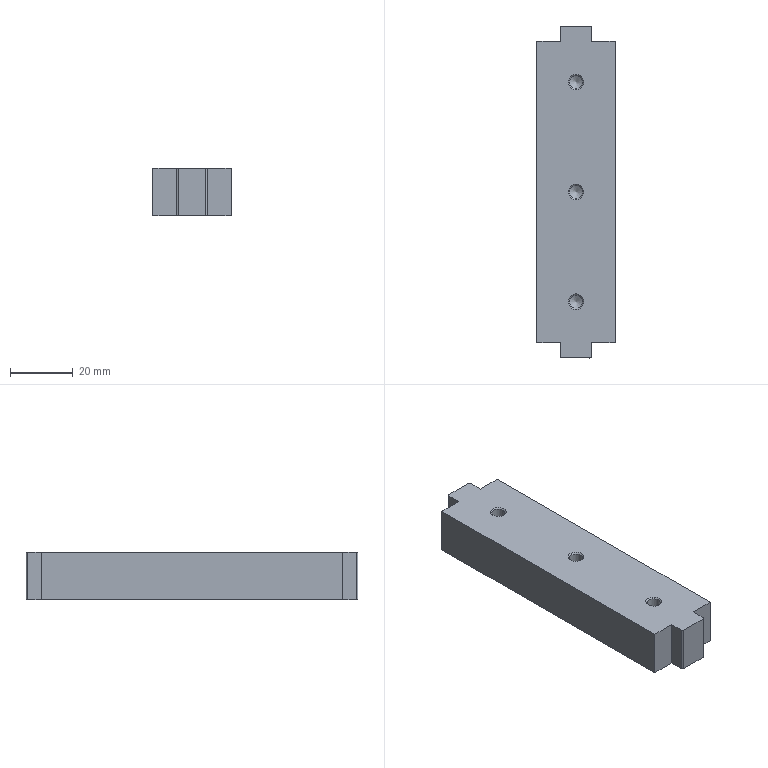Part | STEP file | 200 mesh_id1990 | 1 solid | 27 faces | box 25 x 105.8 x 15 mm | volume 37116 mm3 | plane 14 | cylinder 7 | cone 6 | commonest cylinder face diameters 0.9 x4 4.2 x3
STEP:
#1=CARTESIAN_POINT('',(-17200.384,-3974.819,45.));
#2=VERTEX_POINT('',#1);
#3=CARTESIAN_POINT('',(-17200.384,-4070.819,45.));
#4=VERTEX_POINT('',#3);
#5=CARTESIAN_POINT('',(-17200.384,-4072.469,45.));
#6=DIRECTION('',(0.,-1.,0.));
#7=VECTOR('',#6,1.);
#8=LINE('',#5,#7);
#9=EDGE_CURVE('',#2,#4,#8,.T.);
#10=ORIENTED_EDGE('',*,*,#9,.F.);
#11=CARTESIAN_POINT('',(-17200.384,-3974.819,60.));
#12=VERTEX_POINT('',#11);
#13=CARTESIAN_POINT('',(-17200.384,-3974.819,65.));
#14=DIRECTION('',(0.,0.,-1.));
#15=VECTOR('',#14,1.);
#16=LINE('',#13,#15);
#17=EDGE_CURVE('',#12,#2,#16,.T.);
#18=ORIENTED_EDGE('',*,*,#17,.F.);
#19=CARTESIAN_POINT('',(-17200.384,-4070.819,60.));
#20=VERTEX_POINT('',#19);
#21=CARTESIAN_POINT('',(-17200.384,-3977.669,60.));
#22=DIRECTION('',(0.,-1.,0.));
#23=VECTOR('',#22,1.);
#24=LINE('',#21,#23);
#25=EDGE_CURVE('',#12,#20,#24,.T.);
#26=ORIENTED_EDGE('',*,*,#25,.T.);
#27=CARTESIAN_POINT('',(-17200.384,-4070.819,65.));
#28=DIRECTION('',(0.,0.,-1.));
#29=VECTOR('',#28,1.);
#30=LINE('',#27,#29);
#31=EDGE_CURVE('',#20,#4,#30,.T.);
#32=ORIENTED_EDGE('',*,*,#31,.T.);
#33=EDGE_LOOP('',(#10,#18,#26,#32));
#34=FACE_OUTER_BOUND('',#33,.T.);
#35=CARTESIAN_POINT('',(-17200.384,-3977.669,65.));
#36=DIRECTION('',(1.,0.,0.));
#37=DIRECTION('',(0.,0.,1.));
#38=AXIS2_PLACEMENT_3D('',#35,#36,#37);
#39=PLANE('',#38);
#40=ADVANCED_FACE('',(#34),#39,.T.);
#41=CARTESIAN_POINT('',(-17207.984,-4070.819,45.));
#42=VERTEX_POINT('',#41);
#43=CARTESIAN_POINT('',(-17208.384,-4070.819,45.));
#44=DIRECTION('',(-1.,0.,0.));
#45=VECTOR('',#44,1.);
#46=LINE('',#43,#45);
#47=EDGE_CURVE('',#4,#42,#46,.T.);
#48=ORIENTED_EDGE('',*,*,#47,.F.);
#49=ORIENTED_EDGE('',*,*,#31,.F.);
#50=CARTESIAN_POINT('',(-17207.984,-4070.819,60.));
#51=VERTEX_POINT('',#50);
#52=CARTESIAN_POINT('',(-17208.384,-4070.819,60.));
#53=DIRECTION('',(-1.,0.,0.));
#54=VECTOR('',#53,1.);
#55=LINE('',#52,#54);
#56=EDGE_CURVE('',#20,#51,#55,.T.);
#57=ORIENTED_EDGE('',*,*,#56,.T.);
#58=CARTESIAN_POINT('',(-17207.984,-4070.819,65.));
#59=DIRECTION('',(0.,0.,-1.));
#60=VECTOR('',#59,1.);
#61=LINE('',#58,#60);
#62=EDGE_CURVE('',#51,#42,#61,.T.);
#63=ORIENTED_EDGE('',*,*,#62,.T.);
#64=EDGE_LOOP('',(#48,#49,#57,#63));
#65=FACE_OUTER_BOUND('',#64,.T.);
#66=CARTESIAN_POINT('',(-17200.384,-4070.819,65.));
#67=DIRECTION('',(0.,-1.,0.));
#68=DIRECTION('',(0.,0.,1.));
#69=AXIS2_PLACEMENT_3D('',#66,#67,#68);
#70=PLANE('',#69);
#71=ADVANCED_FACE('',(#65),#70,.T.);
#72=CARTESIAN_POINT('',(-17207.984,-4075.269,45.));
#73=VERTEX_POINT('',#72);
#74=CARTESIAN_POINT('',(-17207.984,-4075.369,45.));
#75=DIRECTION('',(0.,-1.,0.));
#76=VECTOR('',#75,1.);
#77=LINE('',#74,#76);
#78=EDGE_CURVE('',#42,#73,#77,.T.);
#79=ORIENTED_EDGE('',*,*,#78,.F.);
#80=ORIENTED_EDGE('',*,*,#62,.F.);
#81=CARTESIAN_POINT('',(-17207.984,-4075.269,60.));
#82=VERTEX_POINT('',#81);
#83=CARTESIAN_POINT('',(-17207.984,-4075.369,60.));
#84=DIRECTION('',(0.,-1.,0.));
#85=VECTOR('',#84,1.);
#86=LINE('',#83,#85);
#87=EDGE_CURVE('',#51,#82,#86,.T.);
#88=ORIENTED_EDGE('',*,*,#87,.T.);
#89=CARTESIAN_POINT('',(-17207.984,-4075.269,65.));
#90=DIRECTION('',(0.,0.,-1.));
#91=VECTOR('',#90,1.);
#92=LINE('',#89,#91);
#93=EDGE_CURVE('',#82,#73,#92,.T.);
#94=ORIENTED_EDGE('',*,*,#93,.T.);
#95=EDGE_LOOP('',(#79,#80,#88,#94));
#96=FACE_OUTER_BOUND('',#95,.T.);
#97=CARTESIAN_POINT('',(-17207.984,-4070.869,65.));
#98=DIRECTION('',(1.,0.,0.));
#99=DIRECTION('',(0.,0.,1.));
#100=AXIS2_PLACEMENT_3D('',#97,#98,#99);
#101=PLANE('',#100);
#102=ADVANCED_FACE('',(#96),#101,.T.);
#103=CARTESIAN_POINT('',(-17208.434,-4075.719,45.));
#104=VERTEX_POINT('',#103);
#105=CARTESIAN_POINT('',(-17208.434,-4075.269,45.));
#106=DIRECTION('',(0.,0.,-1.));
#107=DIRECTION('',(-1.,0.,0.));
#108=AXIS2_PLACEMENT_3D('',#105,#106,#107);
#109=CIRCLE('',#108,0.45);
#110=EDGE_CURVE('',#73,#104,#109,.T.);
#111=ORIENTED_EDGE('',*,*,#110,.F.);
#112=ORIENTED_EDGE('',*,*,#93,.F.);
#113=CARTESIAN_POINT('',(-17208.434,-4075.719,60.));
#114=VERTEX_POINT('',#113);
#115=CARTESIAN_POINT('',(-17208.434,-4075.269,60.));
#116=DIRECTION('',(0.,0.,-1.));
#117=DIRECTION('',(-1.,0.,0.));
#118=AXIS2_PLACEMENT_3D('',#115,#116,#117);
#119=CIRCLE('',#118,0.45);
#120=EDGE_CURVE('',#82,#114,#119,.T.);
#121=ORIENTED_EDGE('',*,*,#120,.T.);
#122=CARTESIAN_POINT('',(-17208.434,-4075.719,65.));
#123=DIRECTION('',(0.,0.,-1.));
#124=VECTOR('',#123,1.);
#125=LINE('',#122,#124);
#126=EDGE_CURVE('',#114,#104,#125,.T.);
#127=ORIENTED_EDGE('',*,*,#126,.T.);
#128=EDGE_LOOP('',(#111,#112,#121,#127));
#129=FACE_OUTER_BOUND('',#128,.T.);
#130=CARTESIAN_POINT('',(-17208.434,-4075.269,65.));
#131=DIRECTION('',(0.,0.,-1.));
#132=DIRECTION('',(1.,0.,0.));
#133=AXIS2_PLACEMENT_3D('',#130,#131,#132);
#134=CYLINDRICAL_SURFACE('',#133,0.45);
#135=ADVANCED_FACE('',(#129),#134,.T.);
#136=CARTESIAN_POINT('',(-17217.334,-4075.719,45.));
#137=VERTEX_POINT('',#136);
#138=CARTESIAN_POINT('',(-17208.384,-4075.719,45.));
#139=DIRECTION('',(-1.,0.,0.));
#140=VECTOR('',#139,1.);
#141=LINE('',#138,#140);
#142=EDGE_CURVE('',#104,#137,#141,.T.);
#143=ORIENTED_EDGE('',*,*,#142,.F.);
#144=ORIENTED_EDGE('',*,*,#126,.F.);
#145=CARTESIAN_POINT('',(-17217.334,-4075.719,60.));
#146=VERTEX_POINT('',#145);
#147=CARTESIAN_POINT('',(-17208.384,-4075.719,60.));
#148=DIRECTION('',(-1.,0.,0.));
#149=VECTOR('',#148,1.);
#150=LINE('',#147,#149);
#151=EDGE_CURVE('',#114,#146,#150,.T.);
#152=ORIENTED_EDGE('',*,*,#151,.T.);
#153=CARTESIAN_POINT('',(-17217.334,-4075.719,65.));
#154=DIRECTION('',(0.,0.,-1.));
#155=VECTOR('',#154,1.);
#156=LINE('',#153,#155);
#157=EDGE_CURVE('',#146,#137,#156,.T.);
#158=ORIENTED_EDGE('',*,*,#157,.T.);
#159=EDGE_LOOP('',(#143,#144,#152,#158));
#160=FACE_OUTER_BOUND('',#159,.T.);
#161=CARTESIAN_POINT('',(-17208.384,-4075.719,65.));
#162=DIRECTION('',(0.,-1.,0.));
#163=DIRECTION('',(0.,0.,1.));
#164=AXIS2_PLACEMENT_3D('',#161,#162,#163);
#165=PLANE('',#164);
#166=ADVANCED_FACE('',(#160),#165,.T.);
#167=CARTESIAN_POINT('',(-17217.784,-4075.269,45.));
#168=VERTEX_POINT('',#167);
#169=CARTESIAN_POINT('',(-17217.334,-4075.269,45.));
#170=DIRECTION('',(0.,0.,-1.));
#171=DIRECTION('',(-1.,0.,0.));
#172=AXIS2_PLACEMENT_3D('',#169,#170,#171);
#173=CIRCLE('',#172,0.45);
#174=EDGE_CURVE('',#137,#168,#173,.T.);
#175=ORIENTED_EDGE('',*,*,#174,.F.);
#176=ORIENTED_EDGE('',*,*,#157,.F.);
#177=CARTESIAN_POINT('',(-17217.784,-4075.269,60.));
#178=VERTEX_POINT('',#177);
#179=CARTESIAN_POINT('',(-17217.334,-4075.269,60.));
#180=DIRECTION('',(0.,0.,-1.));
#181=DIRECTION('',(-1.,0.,0.));
#182=AXIS2_PLACEMENT_3D('',#179,#180,#181);
#183=CIRCLE('',#182,0.45);
#184=EDGE_CURVE('',#146,#178,#183,.T.);
#185=ORIENTED_EDGE('',*,*,#184,.T.);
#186=CARTESIAN_POINT('',(-17217.784,-4075.269,65.));
#187=DIRECTION('',(0.,0.,-1.));
#188=VECTOR('',#187,1.);
#189=LINE('',#186,#188);
#190=EDGE_CURVE('',#178,#168,#189,.T.);
#191=ORIENTED_EDGE('',*,*,#190,.T.);
#192=EDGE_LOOP('',(#175,#176,#185,#191));
#193=FACE_OUTER_BOUND('',#192,.T.);
#194=CARTESIAN_POINT('',(-17217.334,-4075.269,65.));
#195=DIRECTION('',(0.,0.,-1.));
#196=DIRECTION('',(1.,0.,0.));
#197=AXIS2_PLACEMENT_3D('',#194,#195,#196);
#198=CYLINDRICAL_SURFACE('',#197,0.45);
#199=ADVANCED_FACE('',(#193),#198,.T.);
#200=CARTESIAN_POINT('',(-17217.784,-4070.819,45.));
#201=VERTEX_POINT('',#200);
#202=CARTESIAN_POINT('',(-17217.784,-4075.369,45.));
#203=DIRECTION('',(0.,1.,0.));
#204=VECTOR('',#203,1.);
#205=LINE('',#202,#204);
#206=EDGE_CURVE('',#168,#201,#205,.T.);
#207=ORIENTED_EDGE('',*,*,#206,.F.);
#208=ORIENTED_EDGE('',*,*,#190,.F.);
#209=CARTESIAN_POINT('',(-17217.784,-4070.819,60.));
#210=VERTEX_POINT('',#209);
#211=CARTESIAN_POINT('',(-17217.784,-4075.369,60.));
#212=DIRECTION('',(0.,1.,0.));
#213=VECTOR('',#212,1.);
#214=LINE('',#211,#213);
#215=EDGE_CURVE('',#178,#210,#214,.T.);
#216=ORIENTED_EDGE('',*,*,#215,.T.);
#217=CARTESIAN_POINT('',(-17217.784,-4070.819,65.));
#218=DIRECTION('',(0.,0.,-1.));
#219=VECTOR('',#218,1.);
#220=LINE('',#217,#219);
#221=EDGE_CURVE('',#210,#201,#220,.T.);
#222=ORIENTED_EDGE('',*,*,#221,.T.);
#223=EDGE_LOOP('',(#207,#208,#216,#222));
#224=FACE_OUTER_BOUND('',#223,.T.);
#225=CARTESIAN_POINT('',(-17217.784,-4075.369,65.));
#226=DIRECTION('',(-1.,0.,0.));
#227=DIRECTION('',(0.,0.,-1.));
#228=AXIS2_PLACEMENT_3D('',#225,#226,#227);
#229=PLANE('',#228);
#230=ADVANCED_FACE('',(#224),#229,.T.);
#231=CARTESIAN_POINT('',(-17225.384,-4070.819,45.));
#232=VERTEX_POINT('',#231);
#233=CARTESIAN_POINT('',(-17208.384,-4070.819,45.));
#234=DIRECTION('',(-1.,0.,0.));
#235=VECTOR('',#234,1.);
#236=LINE('',#233,#235);
#237=EDGE_CURVE('',#201,#232,#236,.T.);
#238=ORIENTED_EDGE('',*,*,#237,.F.);
#239=ORIENTED_EDGE('',*,*,#221,.F.);
#240=CARTESIAN_POINT('',(-17225.384,-4070.819,60.));
#241=VERTEX_POINT('',#240);
#242=CARTESIAN_POINT('',(-17208.384,-4070.819,60.));
#243=DIRECTION('',(-1.,0.,0.));
#244=VECTOR('',#243,1.);
#245=LINE('',#242,#244);
#246=EDGE_CURVE('',#210,#241,#245,.T.);
#247=ORIENTED_EDGE('',*,*,#246,.T.);
#248=CARTESIAN_POINT('',(-17225.384,-4070.819,65.));
#249=DIRECTION('',(0.,0.,-1.));
#250=VECTOR('',#249,1.);
#251=LINE('',#248,#250);
#252=EDGE_CURVE('',#241,#232,#251,.T.);
#253=ORIENTED_EDGE('',*,*,#252,.T.);
#254=EDGE_LOOP('',(#238,#239,#247,#253));
#255=FACE_OUTER_BOUND('',#254,.T.);
#256=CARTESIAN_POINT('',(-17217.884,-4070.819,65.));
#257=DIRECTION('',(0.,-1.,0.));
#258=DIRECTION('',(0.,0.,1.));
#259=AXIS2_PLACEMENT_3D('',#256,#257,#258);
#260=PLANE('',#259);
#261=ADVANCED_FACE('',(#255),#260,.T.);
#262=CARTESIAN_POINT('',(-17225.384,-3974.819,45.));
#263=VERTEX_POINT('',#262);
#264=CARTESIAN_POINT('',(-17225.384,-4072.469,45.));
#265=DIRECTION('',(0.,1.,0.));
#266=VECTOR('',#265,1.);
#267=LINE('',#264,#266);
#268=EDGE_CURVE('',#232,#263,#267,.T.);
#269=ORIENTED_EDGE('',*,*,#268,.F.);
#270=ORIENTED_EDGE('',*,*,#252,.F.);
#271=CARTESIAN_POINT('',(-17225.384,-3974.819,60.));
#272=VERTEX_POINT('',#271);
#273=CARTESIAN_POINT('',(-17225.384,-4067.969,60.));
#274=DIRECTION('',(0.,1.,0.));
#275=VECTOR('',#274,1.);
#276=LINE('',#273,#275);
#277=EDGE_CURVE('',#241,#272,#276,.T.);
#278=ORIENTED_EDGE('',*,*,#277,.T.);
#279=CARTESIAN_POINT('',(-17225.384,-3974.819,65.));
#280=DIRECTION('',(0.,0.,-1.));
#281=VECTOR('',#280,1.);
#282=LINE('',#279,#281);
#283=EDGE_CURVE('',#272,#263,#282,.T.);
#284=ORIENTED_EDGE('',*,*,#283,.T.);
#285=EDGE_LOOP('',(#269,#270,#278,#284));
#286=FACE_OUTER_BOUND('',#285,.T.);
#287=CARTESIAN_POINT('',(-17225.384,-4067.969,65.));
#288=DIRECTION('',(-1.,0.,0.));
#289=DIRECTION('',(0.,1.,0.));
#290=AXIS2_PLACEMENT_3D('',#287,#288,#289);
#291=PLANE('',#290);
#292=ADVANCED_FACE('',(#286),#291,.T.);
#293=CARTESIAN_POINT('',(-17217.784,-3974.819,45.));
#294=VERTEX_POINT('',#293);
#295=CARTESIAN_POINT('',(-17208.384,-3974.819,45.));
#296=DIRECTION('',(1.,0.,0.));
#297=VECTOR('',#296,1.);
#298=LINE('',#295,#297);
#299=EDGE_CURVE('',#263,#294,#298,.T.);
#300=ORIENTED_EDGE('',*,*,#299,.F.);
#301=ORIENTED_EDGE('',*,*,#283,.F.);
#302=CARTESIAN_POINT('',(-17217.784,-3974.819,60.));
#303=VERTEX_POINT('',#302);
#304=CARTESIAN_POINT('',(-17208.384,-3974.819,60.));
#305=DIRECTION('',(1.,0.,0.));
#306=VECTOR('',#305,1.);
#307=LINE('',#304,#306);
#308=EDGE_CURVE('',#272,#303,#307,.T.);
#309=ORIENTED_EDGE('',*,*,#308,.T.);
#310=CARTESIAN_POINT('',(-17217.784,-3974.819,65.));
#311=DIRECTION('',(0.,0.,-1.));
#312=VECTOR('',#311,1.);
#313=LINE('',#310,#312);
#314=EDGE_CURVE('',#303,#294,#313,.T.);
#315=ORIENTED_EDGE('',*,*,#314,.T.);
#316=EDGE_LOOP('',(#300,#301,#309,#315));
#317=FACE_OUTER_BOUND('',#316,.T.);
#318=CARTESIAN_POINT('',(-17225.384,-3974.819,65.));
#319=DIRECTION('',(0.,1.,0.));
#320=DIRECTION('',(0.,0.,-1.));
#321=AXIS2_PLACEMENT_3D('',#318,#319,#320);
#322=PLANE('',#321);
#323=ADVANCED_FACE('',(#317),#322,.T.);
#324=CARTESIAN_POINT('',(-17217.784,-3970.369,45.));
#325=VERTEX_POINT('',#324);
#326=CARTESIAN_POINT('',(-17217.784,-4069.569,45.));
#327=DIRECTION('',(0.,1.,0.));
#328=VECTOR('',#327,1.);
#329=LINE('',#326,#328);
#330=EDGE_CURVE('',#294,#325,#329,.T.);
#331=ORIENTED_EDGE('',*,*,#330,.F.);
#332=ORIENTED_EDGE('',*,*,#314,.F.);
#333=CARTESIAN_POINT('',(-17217.784,-3970.369,60.));
#334=VERTEX_POINT('',#333);
#335=CARTESIAN_POINT('',(-17217.784,-4069.569,60.));
#336=DIRECTION('',(0.,1.,0.));
#337=VECTOR('',#336,1.);
#338=LINE('',#335,#337);
#339=EDGE_CURVE('',#303,#334,#338,.T.);
#340=ORIENTED_EDGE('',*,*,#339,.T.);
#341=CARTESIAN_POINT('',(-17217.784,-3970.369,65.));
#342=DIRECTION('',(0.,0.,-1.));
#343=VECTOR('',#342,1.);
#344=LINE('',#341,#343);
#345=EDGE_CURVE('',#334,#325,#344,.T.);
#346=ORIENTED_EDGE('',*,*,#345,.T.);
#347=EDGE_LOOP('',(#331,#332,#340,#346));
#348=FACE_OUTER_BOUND('',#347,.T.);
#349=CARTESIAN_POINT('',(-17217.784,-3974.769,65.));
#350=DIRECTION('',(-1.,0.,0.));
#351=DIRECTION('',(0.,0.,-1.));
#352=AXIS2_PLACEMENT_3D('',#349,#350,#351);
#353=PLANE('',#352);
#354=ADVANCED_FACE('',(#348),#353,.T.);
#355=CARTESIAN_POINT('',(-17217.334,-3969.919,45.));
#356=VERTEX_POINT('',#355);
#357=CARTESIAN_POINT('',(-17217.334,-3970.369,45.));
#358=DIRECTION('',(0.,0.,-1.));
#359=DIRECTION('',(-1.,0.,0.));
#360=AXIS2_PLACEMENT_3D('',#357,#358,#359);
#361=CIRCLE('',#360,0.45);
#362=EDGE_CURVE('',#325,#356,#361,.T.);
#363=ORIENTED_EDGE('',*,*,#362,.F.);
#364=ORIENTED_EDGE('',*,*,#345,.F.);
#365=CARTESIAN_POINT('',(-17217.334,-3969.919,60.));
#366=VERTEX_POINT('',#365);
#367=CARTESIAN_POINT('',(-17217.334,-3970.369,60.));
#368=DIRECTION('',(0.,0.,-1.));
#369=DIRECTION('',(-1.,0.,0.));
#370=AXIS2_PLACEMENT_3D('',#367,#368,#369);
#371=CIRCLE('',#370,0.45);
#372=EDGE_CURVE('',#334,#366,#371,.T.);
#373=ORIENTED_EDGE('',*,*,#372,.T.);
#374=CARTESIAN_POINT('',(-17217.334,-3969.919,65.));
#375=DIRECTION('',(0.,0.,-1.));
#376=VECTOR('',#375,1.);
#377=LINE('',#374,#376);
#378=EDGE_CURVE('',#366,#356,#377,.T.);
#379=ORIENTED_EDGE('',*,*,#378,.T.);
#380=EDGE_LOOP('',(#363,#364,#373,#379));
#381=FACE_OUTER_BOUND('',#380,.T.);
#382=CARTESIAN_POINT('',(-17217.334,-3970.369,65.));
#383=DIRECTION('',(0.,0.,-1.));
#384=DIRECTION('',(1.,0.,0.));
#385=AXIS2_PLACEMENT_3D('',#382,#383,#384);
#386=CYLINDRICAL_SURFACE('',#385,0.45);
#387=ADVANCED_FACE('',(#381),#386,.T.);
#388=CARTESIAN_POINT('',(-17208.434,-3969.919,45.));
#389=VERTEX_POINT('',#388);
#390=CARTESIAN_POINT('',(-17208.384,-3969.919,45.));
#391=DIRECTION('',(1.,0.,0.));
#392=VECTOR('',#391,1.);
#393=LINE('',#390,#392);
#394=EDGE_CURVE('',#356,#389,#393,.T.);
#395=ORIENTED_EDGE('',*,*,#394,.F.);
#396=ORIENTED_EDGE('',*,*,#378,.F.);
#397=CARTESIAN_POINT('',(-17208.434,-3969.919,60.));
#398=VERTEX_POINT('',#397);
#399=CARTESIAN_POINT('',(-17208.384,-3969.919,60.));
#400=DIRECTION('',(1.,0.,0.));
#401=VECTOR('',#400,1.);
#402=LINE('',#399,#401);
#403=EDGE_CURVE('',#366,#398,#402,.T.);
#404=ORIENTED_EDGE('',*,*,#403,.T.);
#405=CARTESIAN_POINT('',(-17208.434,-3969.919,65.));
#406=DIRECTION('',(0.,0.,-1.));
#407=VECTOR('',#406,1.);
#408=LINE('',#405,#407);
#409=EDGE_CURVE('',#398,#389,#408,.T.);
#410=ORIENTED_EDGE('',*,*,#409,.T.);
#411=EDGE_LOOP('',(#395,#396,#404,#410));
#412=FACE_OUTER_BOUND('',#411,.T.);
#413=CARTESIAN_POINT('',(-17217.384,-3969.919,65.));
#414=DIRECTION('',(0.,1.,0.));
#415=DIRECTION('',(0.,0.,-1.));
#416=AXIS2_PLACEMENT_3D('',#413,#414,#415);
#417=PLANE('',#416);
#418=ADVANCED_FACE('',(#412),#417,.T.);
#419=CARTESIAN_POINT('',(-17207.984,-3970.369,45.));
#420=VERTEX_POINT('',#419);
#421=CARTESIAN_POINT('',(-17208.434,-3970.369,45.));
#422=DIRECTION('',(0.,0.,-1.));
#423=DIRECTION('',(-1.,0.,0.));
#424=AXIS2_PLACEMENT_3D('',#421,#422,#423);
#425=CIRCLE('',#424,0.45);
#426=EDGE_CURVE('',#389,#420,#425,.T.);
#427=ORIENTED_EDGE('',*,*,#426,.F.);
#428=ORIENTED_EDGE('',*,*,#409,.F.);
#429=CARTESIAN_POINT('',(-17207.984,-3970.369,60.));
#430=VERTEX_POINT('',#429);
#431=CARTESIAN_POINT('',(-17208.434,-3970.369,60.));
#432=DIRECTION('',(0.,0.,-1.));
#433=DIRECTION('',(-1.,0.,0.));
#434=AXIS2_PLACEMENT_3D('',#431,#432,#433);
#435=CIRCLE('',#434,0.45);
#436=EDGE_CURVE('',#398,#430,#435,.T.);
#437=ORIENTED_EDGE('',*,*,#436,.T.);
#438=CARTESIAN_POINT('',(-17207.984,-3970.369,65.));
#439=DIRECTION('',(0.,0.,-1.));
#440=VECTOR('',#439,1.);
#441=LINE('',#438,#440);
#442=EDGE_CURVE('',#430,#420,#441,.T.);
#443=ORIENTED_EDGE('',*,*,#442,.T.);
#444=EDGE_LOOP('',(#427,#428,#437,#443));
#445=FACE_OUTER_BOUND('',#444,.T.);
#446=CARTESIAN_POINT('',(-17208.434,-3970.369,65.));
#447=DIRECTION('',(0.,0.,-1.));
#448=DIRECTION('',(1.,0.,0.));
#449=AXIS2_PLACEMENT_3D('',#446,#447,#448);
#450=CYLINDRICAL_SURFACE('',#449,0.45);
#451=ADVANCED_FACE('',(#445),#450,.T.);
#452=CARTESIAN_POINT('',(-17207.984,-3974.819,45.));
#453=VERTEX_POINT('',#452);
#454=CARTESIAN_POINT('',(-17207.984,-4069.569,45.));
#455=DIRECTION('',(0.,-1.,0.));
#456=VECTOR('',#455,1.);
#457=LINE('',#454,#456);
#458=EDGE_CURVE('',#420,#453,#457,.T.);
#459=ORIENTED_EDGE('',*,*,#458,.F.);
#460=ORIENTED_EDGE('',*,*,#442,.F.);
#461=CARTESIAN_POINT('',(-17207.984,-3974.819,60.));
#462=VERTEX_POINT('',#461);
#463=CARTESIAN_POINT('',(-17207.984,-4069.569,60.));
#464=DIRECTION('',(0.,-1.,0.));
#465=VECTOR('',#464,1.);
#466=LINE('',#463,#465);
#467=EDGE_CURVE('',#430,#462,#466,.T.);
#468=ORIENTED_EDGE('',*,*,#467,.T.);
#469=CARTESIAN_POINT('',(-17207.984,-3974.819,65.));
#470=DIRECTION('',(0.,0.,-1.));
#471=VECTOR('',#470,1.);
#472=LINE('',#469,#471);
#473=EDGE_CURVE('',#462,#453,#472,.T.);
#474=ORIENTED_EDGE('',*,*,#473,.T.);
#475=EDGE_LOOP('',(#459,#460,#468,#474));
#476=FACE_OUTER_BOUND('',#475,.T.);
#477=CARTESIAN_POINT('',(-17207.984,-3970.269,65.));
#478=DIRECTION('',(1.,0.,0.));
#479=DIRECTION('',(0.,0.,1.));
#480=AXIS2_PLACEMENT_3D('',#477,#478,#479);
#481=PLANE('',#480);
#482=ADVANCED_FACE('',(#476),#481,.T.);
#483=CARTESIAN_POINT('',(-17208.384,-3974.819,45.));
#484=DIRECTION('',(1.,0.,0.));
#485=VECTOR('',#484,1.);
#486=LINE('',#483,#485);
#487=EDGE_CURVE('',#453,#2,#486,.T.);
#488=ORIENTED_EDGE('',*,*,#487,.F.);
#489=ORIENTED_EDGE('',*,*,#473,.F.);
#490=CARTESIAN_POINT('',(-17208.384,-3974.819,60.));
#491=DIRECTION('',(1.,0.,0.));
#492=VECTOR('',#491,1.);
#493=LINE('',#490,#492);
#494=EDGE_CURVE('',#462,#12,#493,.T.);
#495=ORIENTED_EDGE('',*,*,#494,.T.);
#496=ORIENTED_EDGE('',*,*,#17,.T.);
#497=EDGE_LOOP('',(#488,#489,#495,#496));
#498=FACE_OUTER_BOUND('',#497,.T.);
#499=CARTESIAN_POINT('',(-17207.884,-3974.819,65.));
#500=DIRECTION('',(0.,1.,0.));
#501=DIRECTION('',(0.,0.,-1.));
#502=AXIS2_PLACEMENT_3D('',#499,#500,#501);
#503=PLANE('',#502);
#504=ADVANCED_FACE('',(#498),#503,.T.);
#505=CARTESIAN_POINT('',(-17215.384,-4057.819,60.));
#506=VERTEX_POINT('',#505);
#507=CARTESIAN_POINT('',(-17212.884,-4057.819,60.));
#508=DIRECTION('',(0.,0.,-1.));
#509=DIRECTION('',(-1.,0.,0.));
#510=AXIS2_PLACEMENT_3D('',#507,#508,#509);
#511=CIRCLE('',#510,2.5);
#512=EDGE_CURVE('',#506,#506,#511,.T.);
#513=ORIENTED_EDGE('',*,*,#512,.T.);
#514=EDGE_LOOP('',(#513));
#515=FACE_BOUND('',#514,.T.);
#516=CARTESIAN_POINT('',(-17215.384,-4022.819,60.));
#517=VERTEX_POINT('',#516);
#518=CARTESIAN_POINT('',(-17212.884,-4022.819,60.));
#519=DIRECTION('',(0.,0.,-1.));
#520=DIRECTION('',(-1.,0.,0.));
#521=AXIS2_PLACEMENT_3D('',#518,#519,#520);
#522=CIRCLE('',#521,2.5);
#523=EDGE_CURVE('',#517,#517,#522,.T.);
#524=ORIENTED_EDGE('',*,*,#523,.T.);
#525=EDGE_LOOP('',(#524));
#526=FACE_BOUND('',#525,.T.);
#527=CARTESIAN_POINT('',(-17215.384,-3987.819,60.));
#528=VERTEX_POINT('',#527);
#529=CARTESIAN_POINT('',(-17212.884,-3987.819,60.));
#530=DIRECTION('',(0.,0.,-1.));
#531=DIRECTION('',(-1.,0.,0.));
#532=AXIS2_PLACEMENT_3D('',#529,#530,#531);
#533=CIRCLE('',#532,2.5);
#534=EDGE_CURVE('',#528,#528,#533,.T.);
#535=ORIENTED_EDGE('',*,*,#534,.T.);
#536=EDGE_LOOP('',(#535));
#537=FACE_BOUND('',#536,.T.);
#538=ORIENTED_EDGE('',*,*,#25,.F.);
#539=ORIENTED_EDGE('',*,*,#494,.F.);
#540=ORIENTED_EDGE('',*,*,#467,.F.);
#541=ORIENTED_EDGE('',*,*,#436,.F.);
#542=ORIENTED_EDGE('',*,*,#403,.F.);
#543=ORIENTED_EDGE('',*,*,#372,.F.);
#544=ORIENTED_EDGE('',*,*,#339,.F.);
#545=ORIENTED_EDGE('',*,*,#308,.F.);
#546=ORIENTED_EDGE('',*,*,#277,.F.);
#547=ORIENTED_EDGE('',*,*,#246,.F.);
#548=ORIENTED_EDGE('',*,*,#215,.F.);
#549=ORIENTED_EDGE('',*,*,#184,.F.);
#550=ORIENTED_EDGE('',*,*,#151,.F.);
#551=ORIENTED_EDGE('',*,*,#120,.F.);
#552=ORIENTED_EDGE('',*,*,#87,.F.);
#553=ORIENTED_EDGE('',*,*,#56,.F.);
#554=EDGE_LOOP('',(#538,#539,#540,#541,#542,#543,#544,#545,#546,#547,#548,#549,#550,#551,#552,#553));
#555=FACE_BOUND('',#554,.T.);
#556=CARTESIAN_POINT('',(-17208.384,-4072.469,60.));
#557=DIRECTION('',(0.,0.,-1.));
#558=DIRECTION('',(1.,0.,0.));
#559=AXIS2_PLACEMENT_3D('',#556,#557,#558);
#560=PLANE('',#559);
#561=ADVANCED_FACE('',(#515,#526,#537,#555),#560,.F.);
#562=ORIENTED_EDGE('',*,*,#9,.T.);
#563=ORIENTED_EDGE('',*,*,#47,.T.);
#564=ORIENTED_EDGE('',*,*,#78,.T.);
#565=ORIENTED_EDGE('',*,*,#110,.T.);
#566=ORIENTED_EDGE('',*,*,#142,.T.);
#567=ORIENTED_EDGE('',*,*,#174,.T.);
#568=ORIENTED_EDGE('',*,*,#206,.T.);
#569=ORIENTED_EDGE('',*,*,#237,.T.);
#570=ORIENTED_EDGE('',*,*,#268,.T.);
#571=ORIENTED_EDGE('',*,*,#299,.T.);
#572=ORIENTED_EDGE('',*,*,#330,.T.);
#573=ORIENTED_EDGE('',*,*,#362,.T.);
#574=ORIENTED_EDGE('',*,*,#394,.T.);
#575=ORIENTED_EDGE('',*,*,#426,.T.);
#576=ORIENTED_EDGE('',*,*,#458,.T.);
#577=ORIENTED_EDGE('',*,*,#487,.T.);
#578=EDGE_LOOP('',(#562,#563,#564,#565,#566,#567,#568,#569,#570,#571,#572,#573,#574,#575,#576,#577));
#579=FACE_OUTER_BOUND('',#578,.T.);
#580=CARTESIAN_POINT('',(-17208.384,-4072.469,45.));
#581=DIRECTION('',(0.,0.,-1.));
#582=DIRECTION('',(1.,0.,0.));
#583=AXIS2_PLACEMENT_3D('',#580,#581,#582);
#584=PLANE('',#583);
#585=ADVANCED_FACE('',(#579),#584,.T.);
#586=CARTESIAN_POINT('',(-17210.784,-3987.819,52.76));
#587=VERTEX_POINT('',#586);
#588=CARTESIAN_POINT('',(-17212.884,-3987.819,52.76));
#589=DIRECTION('',(0.,0.,1.));
#590=DIRECTION('',(1.,0.,0.));
#591=AXIS2_PLACEMENT_3D('',#588,#589,#590);
#592=CIRCLE('',#591,2.1);
#593=EDGE_CURVE('',#587,#587,#592,.T.);
#594=ORIENTED_EDGE('',*,*,#593,.T.);
#595=EDGE_LOOP('',(#594));
#596=FACE_BOUND('',#595,.T.);
#597=CARTESIAN_POINT('',(-17212.884,-3987.819,51.498));
#598=VERTEX_POINT('',#597);
#599=VERTEX_LOOP('',#598);
#600=FACE_BOUND('',#599,.T.);
#601=CARTESIAN_POINT('',(-17212.884,-3987.819,53.));
#602=DIRECTION('',(0.,0.,1.));
#603=DIRECTION('',(-1.,0.,0.));
#604=AXIS2_PLACEMENT_3D('',#601,#602,#603);
#605=CONICAL_SURFACE('',#604,2.5,59.);
#606=ADVANCED_FACE('',(#596,#600),#605,.F.);
#607=CARTESIAN_POINT('',(-17214.984,-3987.819,59.6));
#608=VERTEX_POINT('',#607);
#609=CARTESIAN_POINT('',(-17212.884,-3987.819,59.6));
#610=DIRECTION('',(0.,0.,1.));
#611=DIRECTION('',(-1.,0.,0.));
#612=AXIS2_PLACEMENT_3D('',#609,#610,#611);
#613=CIRCLE('',#612,2.1);
#614=EDGE_CURVE('',#608,#608,#613,.T.);
#615=ORIENTED_EDGE('',*,*,#614,.T.);
#616=EDGE_LOOP('',(#615));
#617=FACE_BOUND('',#616,.T.);
#618=ORIENTED_EDGE('',*,*,#593,.F.);
#619=EDGE_LOOP('',(#618));
#620=FACE_BOUND('',#619,.T.);
#621=CARTESIAN_POINT('',(-17212.884,-3987.819,65.));
#622=DIRECTION('',(0.,0.,-1.));
#623=DIRECTION('',(1.,0.,0.));
#624=AXIS2_PLACEMENT_3D('',#621,#622,#623);
#625=CYLINDRICAL_SURFACE('',#624,2.1);
#626=ADVANCED_FACE('',(#617,#620),#625,.F.);
#627=CARTESIAN_POINT('',(-17210.784,-4022.819,52.76));
#628=VERTEX_POINT('',#627);
#629=CARTESIAN_POINT('',(-17212.884,-4022.819,52.76));
#630=DIRECTION('',(0.,0.,1.));
#631=DIRECTION('',(1.,0.,0.));
#632=AXIS2_PLACEMENT_3D('',#629,#630,#631);
#633=CIRCLE('',#632,2.1);
#634=EDGE_CURVE('',#628,#628,#633,.T.);
#635=ORIENTED_EDGE('',*,*,#634,.T.);
#636=EDGE_LOOP('',(#635));
#637=FACE_BOUND('',#636,.T.);
#638=CARTESIAN_POINT('',(-17212.884,-4022.819,51.498));
#639=VERTEX_POINT('',#638);
#640=VERTEX_LOOP('',#639);
#641=FACE_BOUND('',#640,.T.);
#642=CARTESIAN_POINT('',(-17212.884,-4022.819,53.));
#643=DIRECTION('',(0.,0.,1.));
#644=DIRECTION('',(-1.,0.,0.));
#645=AXIS2_PLACEMENT_3D('',#642,#643,#644);
#646=CONICAL_SURFACE('',#645,2.5,59.);
#647=ADVANCED_FACE('',(#637,#641),#646,.F.);
#648=CARTESIAN_POINT('',(-17214.984,-4022.819,59.6));
#649=VERTEX_POINT('',#648);
#650=CARTESIAN_POINT('',(-17212.884,-4022.819,59.6));
#651=DIRECTION('',(0.,0.,1.));
#652=DIRECTION('',(-1.,0.,0.));
#653=AXIS2_PLACEMENT_3D('',#650,#651,#652);
#654=CIRCLE('',#653,2.1);
#655=EDGE_CURVE('',#649,#649,#654,.T.);
#656=ORIENTED_EDGE('',*,*,#655,.T.);
#657=EDGE_LOOP('',(#656));
#658=FACE_BOUND('',#657,.T.);
#659=ORIENTED_EDGE('',*,*,#634,.F.);
#660=EDGE_LOOP('',(#659));
#661=FACE_BOUND('',#660,.T.);
#662=CARTESIAN_POINT('',(-17212.884,-4022.819,65.));
#663=DIRECTION('',(0.,0.,-1.));
#664=DIRECTION('',(1.,0.,0.));
#665=AXIS2_PLACEMENT_3D('',#662,#663,#664);
#666=CYLINDRICAL_SURFACE('',#665,2.1);
#667=ADVANCED_FACE('',(#658,#661),#666,.F.);
#668=CARTESIAN_POINT('',(-17210.784,-4057.819,52.76));
#669=VERTEX_POINT('',#668);
#670=CARTESIAN_POINT('',(-17212.884,-4057.819,52.76));
#671=DIRECTION('',(0.,0.,1.));
#672=DIRECTION('',(1.,0.,0.));
#673=AXIS2_PLACEMENT_3D('',#670,#671,#672);
#674=CIRCLE('',#673,2.1);
#675=EDGE_CURVE('',#669,#669,#674,.T.);
#676=ORIENTED_EDGE('',*,*,#675,.T.);
#677=EDGE_LOOP('',(#676));
#678=FACE_BOUND('',#677,.T.);
#679=CARTESIAN_POINT('',(-17212.884,-4057.819,51.498));
#680=VERTEX_POINT('',#679);
#681=VERTEX_LOOP('',#680);
#682=FACE_BOUND('',#681,.T.);
#683=CARTESIAN_POINT('',(-17212.884,-4057.819,53.));
#684=DIRECTION('',(0.,0.,1.));
#685=DIRECTION('',(-1.,0.,0.));
#686=AXIS2_PLACEMENT_3D('',#683,#684,#685);
#687=CONICAL_SURFACE('',#686,2.5,59.);
#688=ADVANCED_FACE('',(#678,#682),#687,.F.);
#689=CARTESIAN_POINT('',(-17214.984,-4057.819,59.6));
#690=VERTEX_POINT('',#689);
#691=CARTESIAN_POINT('',(-17212.884,-4057.819,59.6));
#692=DIRECTION('',(0.,0.,1.));
#693=DIRECTION('',(-1.,0.,0.));
#694=AXIS2_PLACEMENT_3D('',#691,#692,#693);
#695=CIRCLE('',#694,2.1);
#696=EDGE_CURVE('',#690,#690,#695,.T.);
#697=ORIENTED_EDGE('',*,*,#696,.T.);
#698=EDGE_LOOP('',(#697));
#699=FACE_BOUND('',#698,.T.);
#700=ORIENTED_EDGE('',*,*,#675,.F.);
#701=EDGE_LOOP('',(#700));
#702=FACE_BOUND('',#701,.T.);
#703=CARTESIAN_POINT('',(-17212.884,-4057.819,65.));
#704=DIRECTION('',(0.,0.,-1.));
#705=DIRECTION('',(1.,0.,0.));
#706=AXIS2_PLACEMENT_3D('',#703,#704,#705);
#707=CYLINDRICAL_SURFACE('',#706,2.1);
#708=ADVANCED_FACE('',(#699,#702),#707,.F.);
#709=ORIENTED_EDGE('',*,*,#696,.F.);
#710=EDGE_LOOP('',(#709));
#711=FACE_BOUND('',#710,.T.);
#712=ORIENTED_EDGE('',*,*,#512,.F.);
#713=EDGE_LOOP('',(#712));
#714=FACE_BOUND('',#713,.T.);
#715=CARTESIAN_POINT('',(-17212.884,-4057.819,60.));
#716=DIRECTION('',(0.,0.,1.));
#717=DIRECTION('',(-1.,0.,0.));
#718=AXIS2_PLACEMENT_3D('',#715,#716,#717);
#719=CONICAL_SURFACE('',#718,2.5,45.);
#720=ADVANCED_FACE('',(#711,#714),#719,.F.);
#721=ORIENTED_EDGE('',*,*,#655,.F.);
#722=EDGE_LOOP('',(#721));
#723=FACE_BOUND('',#722,.T.);
#724=ORIENTED_EDGE('',*,*,#523,.F.);
#725=EDGE_LOOP('',(#724));
#726=FACE_BOUND('',#725,.T.);
#727=CARTESIAN_POINT('',(-17212.884,-4022.819,60.));
#728=DIRECTION('',(0.,0.,1.));
#729=DIRECTION('',(-1.,0.,0.));
#730=AXIS2_PLACEMENT_3D('',#727,#728,#729);
#731=CONICAL_SURFACE('',#730,2.5,45.);
#732=ADVANCED_FACE('',(#723,#726),#731,.F.);
#733=ORIENTED_EDGE('',*,*,#614,.F.);
#734=EDGE_LOOP('',(#733));
#735=FACE_BOUND('',#734,.T.);
#736=ORIENTED_EDGE('',*,*,#534,.F.);
#737=EDGE_LOOP('',(#736));
#738=FACE_BOUND('',#737,.T.);
#739=CARTESIAN_POINT('',(-17212.884,-3987.819,60.));
#740=DIRECTION('',(0.,0.,1.));
#741=DIRECTION('',(-1.,0.,0.));
#742=AXIS2_PLACEMENT_3D('',#739,#740,#741);
#743=CONICAL_SURFACE('',#742,2.5,45.);
#744=ADVANCED_FACE('',(#735,#738),#743,.F.);
#745=CLOSED_SHELL('',(#40,#71,#102,#135,#166,#199,#230,#261,#292,#323,#354,#387,#418,#451,#482,#504,#561,#585,#606,#626,#647,#667,#688,#708,#720,#732,#744));
#746=MANIFOLD_SOLID_BREP('',#745);
#747=(LENGTH_UNIT()NAMED_UNIT(*)SI_UNIT(.MILLI.,.METRE.));
#748=UNCERTAINTY_MEASURE_WITH_UNIT(LENGTH_MEASURE(0.00002),#747,'','');
#749=(NAMED_UNIT(*)PLANE_ANGLE_UNIT()SI_UNIT($,.RADIAN.));
#750=PLANE_ANGLE_MEASURE_WITH_UNIT(PLANE_ANGLE_MEASURE(0.01745),#749);
#751=DIMENSIONAL_EXPONENTS(0.,0.,0.,0.,0.,0.,0.);
#752=(CONVERSION_BASED_UNIT('DEGREE',#750)NAMED_UNIT(#751)PLANE_ANGLE_UNIT());
#753=(NAMED_UNIT(*)SI_UNIT($,.STERADIAN.)SOLID_ANGLE_UNIT());
#754=(GEOMETRIC_REPRESENTATION_CONTEXT(3)GLOBAL_UNCERTAINTY_ASSIGNED_CONTEXT((#748))GLOBAL_UNIT_ASSIGNED_CONTEXT((#747,#752,#753))REPRESENTATION_CONTEXT('',''));
#755=ADVANCED_BREP_SHAPE_REPRESENTATION('',(#746),#754);